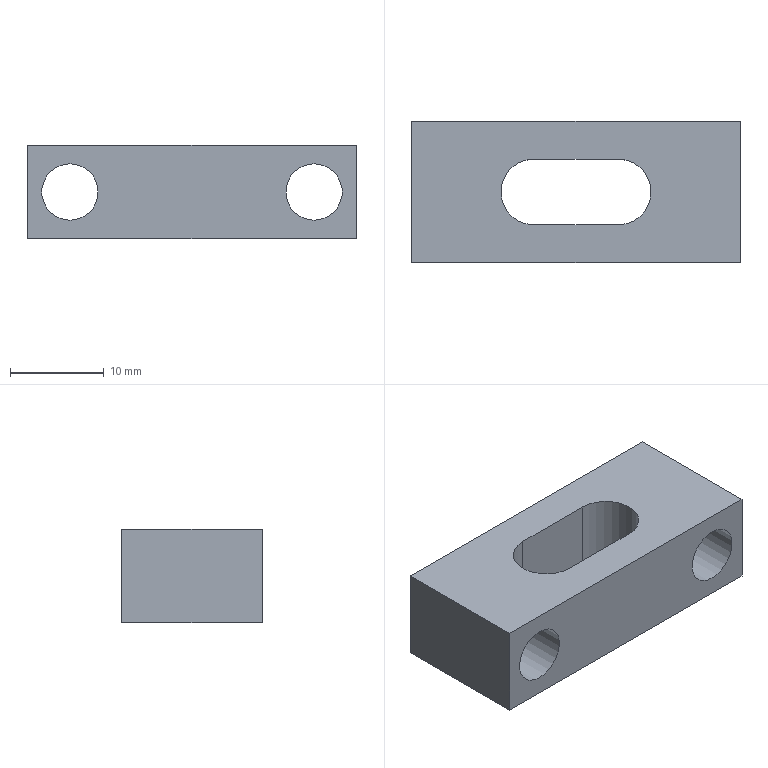Part | NX | features BREP 1 | 1 solid | 12 faces | box 35 x 15 x 10 mm | volume 3387 mm3 | plane 8 | cylinder 4 | commonest cylinder face diameters 6 x2 7 x2
STEP:
#1=CARTESIAN_POINT('',(17.5,-7.5,-10.));
#2=VERTEX_POINT('',#1);
#3=CARTESIAN_POINT('',(17.5,7.5,-10.));
#4=VERTEX_POINT('',#3);
#5=CARTESIAN_POINT('',(17.5,7.5,-10.));
#6=DIRECTION('',(0.,1.,0.));
#7=VECTOR('',#6,1000.);
#8=LINE('',#5,#7);
#9=EDGE_CURVE('',#2,#4,#8,.T.);
#10=ORIENTED_EDGE('',*,*,#9,.F.);
#11=CARTESIAN_POINT('',(-17.5,-7.5,-10.));
#12=VERTEX_POINT('',#11);
#13=CARTESIAN_POINT('',(-17.5,-7.5,-10.));
#14=DIRECTION('',(1.,0.,0.));
#15=VECTOR('',#14,1000.);
#16=LINE('',#13,#15);
#17=EDGE_CURVE('',#12,#2,#16,.T.);
#18=ORIENTED_EDGE('',*,*,#17,.F.);
#19=CARTESIAN_POINT('',(-17.5,7.5,-10.));
#20=VERTEX_POINT('',#19);
#21=CARTESIAN_POINT('',(-17.5,7.5,-10.));
#22=DIRECTION('',(0.,-1.,0.));
#23=VECTOR('',#22,1000.);
#24=LINE('',#21,#23);
#25=EDGE_CURVE('',#20,#12,#24,.T.);
#26=ORIENTED_EDGE('',*,*,#25,.F.);
#27=CARTESIAN_POINT('',(-17.5,7.5,-10.));
#28=DIRECTION('',(-1.,0.,0.));
#29=VECTOR('',#28,1000.);
#30=LINE('',#27,#29);
#31=EDGE_CURVE('',#4,#20,#30,.T.);
#32=ORIENTED_EDGE('',*,*,#31,.F.);
#33=EDGE_LOOP('',(#10,#18,#26,#32));
#34=FACE_BOUND('',#33,.T.);
#35=CARTESIAN_POINT('',(-4.5,-3.5,-10.));
#36=VERTEX_POINT('',#35);
#37=CARTESIAN_POINT('',(4.5,-3.5,-10.));
#38=VERTEX_POINT('',#37);
#39=CARTESIAN_POINT('',(-4.5,-3.5,-10.));
#40=DIRECTION('',(1.,0.,0.));
#41=VECTOR('',#40,1000.);
#42=LINE('',#39,#41);
#43=EDGE_CURVE('',#36,#38,#42,.T.);
#44=ORIENTED_EDGE('',*,*,#43,.T.);
#45=CARTESIAN_POINT('',(4.5,3.5,-10.));
#46=VERTEX_POINT('',#45);
#47=CARTESIAN_POINT('',(4.5,0.,-10.));
#48=DIRECTION('',(0.,0.,1.));
#49=DIRECTION('',(1.,0.,0.));
#50=AXIS2_PLACEMENT_3D('',#47,#48,#49);
#51=CIRCLE('',#50,3.5);
#52=EDGE_CURVE('',#38,#46,#51,.T.);
#53=ORIENTED_EDGE('',*,*,#52,.T.);
#54=CARTESIAN_POINT('',(-4.5,3.5,-10.));
#55=VERTEX_POINT('',#54);
#56=CARTESIAN_POINT('',(-4.5,3.5,-10.));
#57=DIRECTION('',(-1.,0.,0.));
#58=VECTOR('',#57,1000.);
#59=LINE('',#56,#58);
#60=EDGE_CURVE('',#46,#55,#59,.T.);
#61=ORIENTED_EDGE('',*,*,#60,.T.);
#62=CARTESIAN_POINT('',(-4.5,0.,-10.));
#63=DIRECTION('',(0.,0.,1.));
#64=DIRECTION('',(1.,0.,0.));
#65=AXIS2_PLACEMENT_3D('',#62,#63,#64);
#66=CIRCLE('',#65,3.5);
#67=EDGE_CURVE('',#55,#36,#66,.T.);
#68=ORIENTED_EDGE('',*,*,#67,.T.);
#69=EDGE_LOOP('',(#44,#53,#61,#68));
#70=FACE_BOUND('',#69,.T.);
#71=CARTESIAN_POINT('',(0.,0.,-10.));
#72=DIRECTION('',(0.,0.,-1.));
#73=DIRECTION('',(-1.,0.,0.));
#74=AXIS2_PLACEMENT_3D('',#71,#72,#73);
#75=PLANE('',#74);
#76=ADVANCED_FACE('',(#34,#70),#75,.T.);
#77=CARTESIAN_POINT('',(17.5,-7.5,0.));
#78=VERTEX_POINT('',#77);
#79=CARTESIAN_POINT('',(17.5,7.5,0.));
#80=VERTEX_POINT('',#79);
#81=CARTESIAN_POINT('',(17.5,7.5,0.));
#82=DIRECTION('',(0.,1.,0.));
#83=VECTOR('',#82,1000.);
#84=LINE('',#81,#83);
#85=EDGE_CURVE('',#78,#80,#84,.T.);
#86=ORIENTED_EDGE('',*,*,#85,.T.);
#87=CARTESIAN_POINT('',(-17.5,7.5,0.));
#88=VERTEX_POINT('',#87);
#89=CARTESIAN_POINT('',(-17.5,7.5,0.));
#90=DIRECTION('',(-1.,0.,0.));
#91=VECTOR('',#90,1000.);
#92=LINE('',#89,#91);
#93=EDGE_CURVE('',#80,#88,#92,.T.);
#94=ORIENTED_EDGE('',*,*,#93,.T.);
#95=CARTESIAN_POINT('',(-17.5,-7.5,0.));
#96=VERTEX_POINT('',#95);
#97=CARTESIAN_POINT('',(-17.5,7.5,0.));
#98=DIRECTION('',(0.,-1.,0.));
#99=VECTOR('',#98,1000.);
#100=LINE('',#97,#99);
#101=EDGE_CURVE('',#88,#96,#100,.T.);
#102=ORIENTED_EDGE('',*,*,#101,.T.);
#103=CARTESIAN_POINT('',(-17.5,-7.5,0.));
#104=DIRECTION('',(1.,0.,0.));
#105=VECTOR('',#104,1000.);
#106=LINE('',#103,#105);
#107=EDGE_CURVE('',#96,#78,#106,.T.);
#108=ORIENTED_EDGE('',*,*,#107,.T.);
#109=EDGE_LOOP('',(#86,#94,#102,#108));
#110=FACE_BOUND('',#109,.T.);
#111=CARTESIAN_POINT('',(-4.5,3.5,0.));
#112=VERTEX_POINT('',#111);
#113=CARTESIAN_POINT('',(-4.5,-3.5,0.));
#114=VERTEX_POINT('',#113);
#115=CARTESIAN_POINT('',(-4.5,0.,0.));
#116=DIRECTION('',(0.,0.,1.));
#117=DIRECTION('',(1.,0.,0.));
#118=AXIS2_PLACEMENT_3D('',#115,#116,#117);
#119=CIRCLE('',#118,3.5);
#120=EDGE_CURVE('',#112,#114,#119,.T.);
#121=ORIENTED_EDGE('',*,*,#120,.F.);
#122=CARTESIAN_POINT('',(4.5,3.5,0.));
#123=VERTEX_POINT('',#122);
#124=CARTESIAN_POINT('',(-4.5,3.5,0.));
#125=DIRECTION('',(-1.,0.,0.));
#126=VECTOR('',#125,1000.);
#127=LINE('',#124,#126);
#128=EDGE_CURVE('',#123,#112,#127,.T.);
#129=ORIENTED_EDGE('',*,*,#128,.F.);
#130=CARTESIAN_POINT('',(4.5,-3.5,0.));
#131=VERTEX_POINT('',#130);
#132=CARTESIAN_POINT('',(4.5,0.,0.));
#133=DIRECTION('',(0.,0.,1.));
#134=DIRECTION('',(1.,0.,0.));
#135=AXIS2_PLACEMENT_3D('',#132,#133,#134);
#136=CIRCLE('',#135,3.5);
#137=EDGE_CURVE('',#131,#123,#136,.T.);
#138=ORIENTED_EDGE('',*,*,#137,.F.);
#139=CARTESIAN_POINT('',(-4.5,-3.5,0.));
#140=DIRECTION('',(1.,0.,0.));
#141=VECTOR('',#140,1000.);
#142=LINE('',#139,#141);
#143=EDGE_CURVE('',#114,#131,#142,.T.);
#144=ORIENTED_EDGE('',*,*,#143,.F.);
#145=EDGE_LOOP('',(#121,#129,#138,#144));
#146=FACE_BOUND('',#145,.T.);
#147=CARTESIAN_POINT('',(0.,0.,0.));
#148=DIRECTION('',(0.,0.,-1.));
#149=DIRECTION('',(-1.,0.,0.));
#150=AXIS2_PLACEMENT_3D('',#147,#148,#149);
#151=PLANE('',#150);
#152=ADVANCED_FACE('',(#110,#146),#151,.F.);
#153=ORIENTED_EDGE('',*,*,#85,.F.);
#154=CARTESIAN_POINT('',(17.5,-7.5,-10.));
#155=DIRECTION('',(0.,0.,1.));
#156=VECTOR('',#155,1000.);
#157=LINE('',#154,#156);
#158=EDGE_CURVE('',#2,#78,#157,.T.);
#159=ORIENTED_EDGE('',*,*,#158,.F.);
#160=ORIENTED_EDGE('',*,*,#9,.T.);
#161=CARTESIAN_POINT('',(17.5,7.5,-10.));
#162=DIRECTION('',(0.,0.,1.));
#163=VECTOR('',#162,1000.);
#164=LINE('',#161,#163);
#165=EDGE_CURVE('',#4,#80,#164,.T.);
#166=ORIENTED_EDGE('',*,*,#165,.T.);
#167=EDGE_LOOP('',(#153,#159,#160,#166));
#168=FACE_BOUND('',#167,.T.);
#169=CARTESIAN_POINT('',(17.5,7.5,-10.));
#170=DIRECTION('',(-1.,0.,0.));
#171=DIRECTION('',(0.,1.,0.));
#172=AXIS2_PLACEMENT_3D('',#169,#170,#171);
#173=PLANE('',#172);
#174=ADVANCED_FACE('',(#168),#173,.F.);
#175=CARTESIAN_POINT('',(-13.,7.5,-8.));
#176=VERTEX_POINT('',#175);
#177=CARTESIAN_POINT('',(-13.,7.5,-5.));
#178=DIRECTION('',(0.,-1.,0.));
#179=DIRECTION('',(0.,0.,-1.));
#180=AXIS2_PLACEMENT_3D('',#177,#178,#179);
#181=CIRCLE('',#180,3.);
#182=EDGE_CURVE('',#176,#176,#181,.T.);
#183=ORIENTED_EDGE('',*,*,#182,.T.);
#184=EDGE_LOOP('',(#183));
#185=FACE_BOUND('',#184,.T.);
#186=CARTESIAN_POINT('',(13.,7.5,-8.));
#187=VERTEX_POINT('',#186);
#188=CARTESIAN_POINT('',(13.,7.5,-5.));
#189=DIRECTION('',(0.,-1.,0.));
#190=DIRECTION('',(0.,0.,-1.));
#191=AXIS2_PLACEMENT_3D('',#188,#189,#190);
#192=CIRCLE('',#191,3.);
#193=EDGE_CURVE('',#187,#187,#192,.T.);
#194=ORIENTED_EDGE('',*,*,#193,.T.);
#195=EDGE_LOOP('',(#194));
#196=FACE_BOUND('',#195,.T.);
#197=ORIENTED_EDGE('',*,*,#93,.F.);
#198=ORIENTED_EDGE('',*,*,#165,.F.);
#199=ORIENTED_EDGE('',*,*,#31,.T.);
#200=CARTESIAN_POINT('',(-17.5,7.5,-10.));
#201=DIRECTION('',(0.,0.,1.));
#202=VECTOR('',#201,1000.);
#203=LINE('',#200,#202);
#204=EDGE_CURVE('',#20,#88,#203,.T.);
#205=ORIENTED_EDGE('',*,*,#204,.T.);
#206=EDGE_LOOP('',(#197,#198,#199,#205));
#207=FACE_BOUND('',#206,.T.);
#208=CARTESIAN_POINT('',(-17.5,7.5,-10.));
#209=DIRECTION('',(0.,-1.,0.));
#210=DIRECTION('',(0.,0.,-1.));
#211=AXIS2_PLACEMENT_3D('',#208,#209,#210);
#212=PLANE('',#211);
#213=ADVANCED_FACE('',(#185,#196,#207),#212,.F.);
#214=ORIENTED_EDGE('',*,*,#101,.F.);
#215=ORIENTED_EDGE('',*,*,#204,.F.);
#216=ORIENTED_EDGE('',*,*,#25,.T.);
#217=CARTESIAN_POINT('',(-17.5,-7.5,-10.));
#218=DIRECTION('',(0.,0.,1.));
#219=VECTOR('',#218,1000.);
#220=LINE('',#217,#219);
#221=EDGE_CURVE('',#12,#96,#220,.T.);
#222=ORIENTED_EDGE('',*,*,#221,.T.);
#223=EDGE_LOOP('',(#214,#215,#216,#222));
#224=FACE_BOUND('',#223,.T.);
#225=CARTESIAN_POINT('',(-17.5,7.5,-10.));
#226=DIRECTION('',(1.,0.,0.));
#227=DIRECTION('',(0.,-1.,0.));
#228=AXIS2_PLACEMENT_3D('',#225,#226,#227);
#229=PLANE('',#228);
#230=ADVANCED_FACE('',(#224),#229,.F.);
#231=CARTESIAN_POINT('',(-13.,-7.5,-8.));
#232=VERTEX_POINT('',#231);
#233=CARTESIAN_POINT('',(-13.,-7.5,-5.));
#234=DIRECTION('',(0.,-1.,0.));
#235=DIRECTION('',(0.,0.,-1.));
#236=AXIS2_PLACEMENT_3D('',#233,#234,#235);
#237=CIRCLE('',#236,3.);
#238=EDGE_CURVE('',#232,#232,#237,.T.);
#239=ORIENTED_EDGE('',*,*,#238,.F.);
#240=EDGE_LOOP('',(#239));
#241=FACE_BOUND('',#240,.T.);
#242=CARTESIAN_POINT('',(13.,-7.5,-8.));
#243=VERTEX_POINT('',#242);
#244=CARTESIAN_POINT('',(13.,-7.5,-5.));
#245=DIRECTION('',(0.,-1.,0.));
#246=DIRECTION('',(0.,0.,-1.));
#247=AXIS2_PLACEMENT_3D('',#244,#245,#246);
#248=CIRCLE('',#247,3.);
#249=EDGE_CURVE('',#243,#243,#248,.T.);
#250=ORIENTED_EDGE('',*,*,#249,.F.);
#251=EDGE_LOOP('',(#250));
#252=FACE_BOUND('',#251,.T.);
#253=ORIENTED_EDGE('',*,*,#107,.F.);
#254=ORIENTED_EDGE('',*,*,#221,.F.);
#255=ORIENTED_EDGE('',*,*,#17,.T.);
#256=ORIENTED_EDGE('',*,*,#158,.T.);
#257=EDGE_LOOP('',(#253,#254,#255,#256));
#258=FACE_BOUND('',#257,.T.);
#259=CARTESIAN_POINT('',(-17.5,-7.5,-10.));
#260=DIRECTION('',(0.,1.,0.));
#261=DIRECTION('',(0.,0.,1.));
#262=AXIS2_PLACEMENT_3D('',#259,#260,#261);
#263=PLANE('',#262);
#264=ADVANCED_FACE('',(#241,#252,#258),#263,.F.);
#265=ORIENTED_EDGE('',*,*,#120,.T.);
#266=CARTESIAN_POINT('',(-4.5,-3.5,-10.));
#267=DIRECTION('',(0.,0.,1.));
#268=VECTOR('',#267,1000.);
#269=LINE('',#266,#268);
#270=EDGE_CURVE('',#36,#114,#269,.T.);
#271=ORIENTED_EDGE('',*,*,#270,.F.);
#272=ORIENTED_EDGE('',*,*,#67,.F.);
#273=CARTESIAN_POINT('',(-4.5,3.5,-10.));
#274=DIRECTION('',(0.,0.,1.));
#275=VECTOR('',#274,1000.);
#276=LINE('',#273,#275);
#277=EDGE_CURVE('',#55,#112,#276,.T.);
#278=ORIENTED_EDGE('',*,*,#277,.T.);
#279=EDGE_LOOP('',(#265,#271,#272,#278));
#280=FACE_BOUND('',#279,.T.);
#281=CARTESIAN_POINT('',(-4.5,0.,-10.));
#282=DIRECTION('',(0.,0.,1.));
#283=DIRECTION('',(1.,0.,0.));
#284=AXIS2_PLACEMENT_3D('',#281,#282,#283);
#285=CYLINDRICAL_SURFACE('',#284,3.5);
#286=ADVANCED_FACE('',(#280),#285,.F.);
#287=ORIENTED_EDGE('',*,*,#143,.T.);
#288=CARTESIAN_POINT('',(4.5,-3.5,-10.));
#289=DIRECTION('',(0.,0.,1.));
#290=VECTOR('',#289,1000.);
#291=LINE('',#288,#290);
#292=EDGE_CURVE('',#38,#131,#291,.T.);
#293=ORIENTED_EDGE('',*,*,#292,.F.);
#294=ORIENTED_EDGE('',*,*,#43,.F.);
#295=ORIENTED_EDGE('',*,*,#270,.T.);
#296=EDGE_LOOP('',(#287,#293,#294,#295));
#297=FACE_BOUND('',#296,.T.);
#298=CARTESIAN_POINT('',(-4.5,-3.5,-10.));
#299=DIRECTION('',(0.,1.,0.));
#300=DIRECTION('',(0.,0.,1.));
#301=AXIS2_PLACEMENT_3D('',#298,#299,#300);
#302=PLANE('',#301);
#303=ADVANCED_FACE('',(#297),#302,.T.);
#304=ORIENTED_EDGE('',*,*,#137,.T.);
#305=CARTESIAN_POINT('',(4.5,3.5,-10.));
#306=DIRECTION('',(0.,0.,1.));
#307=VECTOR('',#306,1000.);
#308=LINE('',#305,#307);
#309=EDGE_CURVE('',#46,#123,#308,.T.);
#310=ORIENTED_EDGE('',*,*,#309,.F.);
#311=ORIENTED_EDGE('',*,*,#52,.F.);
#312=ORIENTED_EDGE('',*,*,#292,.T.);
#313=EDGE_LOOP('',(#304,#310,#311,#312));
#314=FACE_BOUND('',#313,.T.);
#315=CARTESIAN_POINT('',(4.5,0.,-10.));
#316=DIRECTION('',(0.,0.,1.));
#317=DIRECTION('',(1.,0.,0.));
#318=AXIS2_PLACEMENT_3D('',#315,#316,#317);
#319=CYLINDRICAL_SURFACE('',#318,3.5);
#320=ADVANCED_FACE('',(#314),#319,.F.);
#321=ORIENTED_EDGE('',*,*,#128,.T.);
#322=ORIENTED_EDGE('',*,*,#277,.F.);
#323=ORIENTED_EDGE('',*,*,#60,.F.);
#324=ORIENTED_EDGE('',*,*,#309,.T.);
#325=EDGE_LOOP('',(#321,#322,#323,#324));
#326=FACE_BOUND('',#325,.T.);
#327=CARTESIAN_POINT('',(-4.5,3.5,-10.));
#328=DIRECTION('',(0.,-1.,0.));
#329=DIRECTION('',(0.,0.,-1.));
#330=AXIS2_PLACEMENT_3D('',#327,#328,#329);
#331=PLANE('',#330);
#332=ADVANCED_FACE('',(#326),#331,.T.);
#333=ORIENTED_EDGE('',*,*,#193,.F.);
#334=EDGE_LOOP('',(#333));
#335=FACE_BOUND('',#334,.T.);
#336=ORIENTED_EDGE('',*,*,#249,.T.);
#337=EDGE_LOOP('',(#336));
#338=FACE_BOUND('',#337,.T.);
#339=CARTESIAN_POINT('',(13.,7.5,-5.));
#340=DIRECTION('',(0.,1.,0.));
#341=DIRECTION('',(0.,0.,1.));
#342=AXIS2_PLACEMENT_3D('',#339,#340,#341);
#343=CYLINDRICAL_SURFACE('',#342,3.);
#344=ADVANCED_FACE('',(#335,#338),#343,.F.);
#345=ORIENTED_EDGE('',*,*,#182,.F.);
#346=EDGE_LOOP('',(#345));
#347=FACE_BOUND('',#346,.T.);
#348=ORIENTED_EDGE('',*,*,#238,.T.);
#349=EDGE_LOOP('',(#348));
#350=FACE_BOUND('',#349,.T.);
#351=CARTESIAN_POINT('',(-13.,7.5,-5.));
#352=DIRECTION('',(0.,1.,0.));
#353=DIRECTION('',(0.,0.,1.));
#354=AXIS2_PLACEMENT_3D('',#351,#352,#353);
#355=CYLINDRICAL_SURFACE('',#354,3.);
#356=ADVANCED_FACE('',(#347,#350),#355,.F.);
#357=CLOSED_SHELL('',(#76,#152,#174,#213,#230,#264,#286,#303,#320,#332,#344,#356));
#358=MANIFOLD_SOLID_BREP('',#357);
#359=(LENGTH_UNIT()NAMED_UNIT(*)SI_UNIT(.MILLI.,.METRE.));
#360=UNCERTAINTY_MEASURE_WITH_UNIT(LENGTH_MEASURE(0.00001),#359,'','');
#361=(NAMED_UNIT(*)PLANE_ANGLE_UNIT()SI_UNIT($,.RADIAN.));
#362=(NAMED_UNIT(*)SI_UNIT($,.STERADIAN.)SOLID_ANGLE_UNIT());
#363=(GEOMETRIC_REPRESENTATION_CONTEXT(3)GLOBAL_UNCERTAINTY_ASSIGNED_CONTEXT((#360))GLOBAL_UNIT_ASSIGNED_CONTEXT((#359,#361,#362))REPRESENTATION_CONTEXT('',''));
#364=ADVANCED_BREP_SHAPE_REPRESENTATION('',(#358),#363);